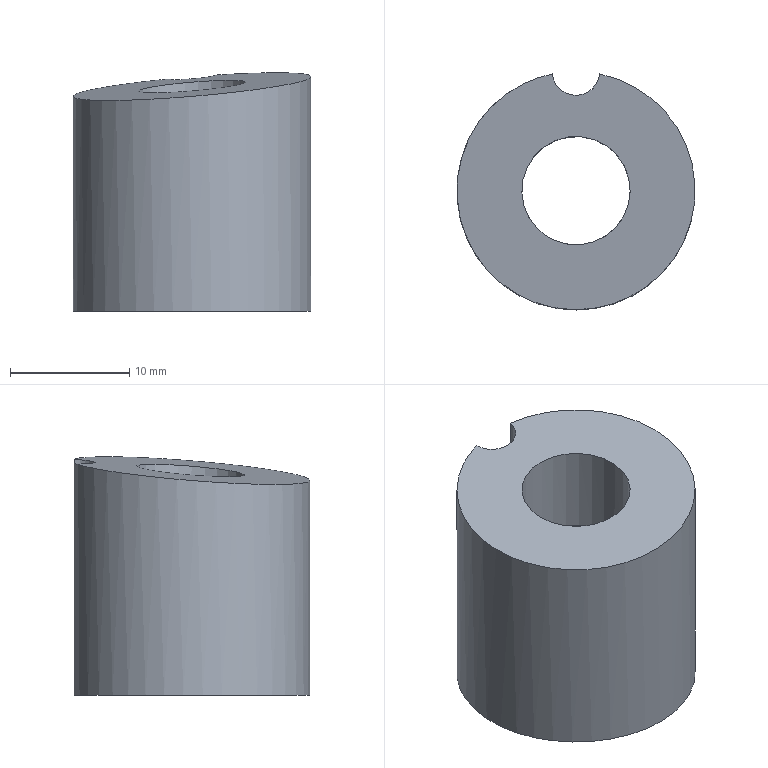Part | NX | features EKSD 20-20-10.10 2 | 1 solid | 7 faces | box 20 x 19.8 x 20.027 mm | volume 3866 mm3 | cylinder 4 | plane 3 | commonest cylinder face diameters 4 x1 9.1 x1 12.6 x1 20 x1
STEP:
#1=CARTESIAN_POINT('',(716.324,18.77,-15.));
#2=VERTEX_POINT('',#1);
#3=CARTESIAN_POINT('',(720.304,18.77,-15.));
#4=VERTEX_POINT('',#3);
#5=CARTESIAN_POINT('',(718.314,18.97,-15.));
#6=DIRECTION('',(0.,0.,1.));
#7=DIRECTION('',(1.,0.,0.));
#8=AXIS2_PLACEMENT_3D('',#5,#6,#7);
#9=CIRCLE('',#8,2.);
#10=EDGE_CURVE('',#2,#4,#9,.T.);
#11=ORIENTED_EDGE('',*,*,#10,.T.);
#12=CARTESIAN_POINT('',(718.314,8.97,-15.));
#13=DIRECTION('',(0.,0.,1.));
#14=DIRECTION('',(1.,0.,0.));
#15=AXIS2_PLACEMENT_3D('',#12,#13,#14);
#16=CIRCLE('',#15,10.);
#17=EDGE_CURVE('',#2,#4,#16,.T.);
#18=ORIENTED_EDGE('',*,*,#17,.F.);
#19=EDGE_LOOP('',(#11,#18));
#20=FACE_BOUND('',#19,.T.);
#21=CARTESIAN_POINT('',(712.014,8.97,-15.));
#22=VERTEX_POINT('',#21);
#23=CARTESIAN_POINT('',(718.314,8.97,-15.));
#24=DIRECTION('',(0.,0.,-1.));
#25=DIRECTION('',(-1.,0.,0.));
#26=AXIS2_PLACEMENT_3D('',#23,#24,#25);
#27=CIRCLE('',#26,6.3);
#28=EDGE_CURVE('',#22,#22,#27,.T.);
#29=ORIENTED_EDGE('',*,*,#28,.F.);
#30=EDGE_LOOP('',(#29));
#31=FACE_BOUND('',#30,.T.);
#32=CARTESIAN_POINT('',(718.314,8.97,-15.));
#33=DIRECTION('',(0.,0.,-1.));
#34=DIRECTION('',(-1.,0.,0.));
#35=AXIS2_PLACEMENT_3D('',#32,#33,#34);
#36=PLANE('',#35);
#37=ADVANCED_FACE('',(#20,#31),#36,.T.);
#38=CARTESIAN_POINT('',(720.304,18.77,4.83));
#39=VERTEX_POINT('',#38);
#40=CARTESIAN_POINT('',(716.324,18.77,4.501));
#41=VERTEX_POINT('',#40);
#42=CARTESIAN_POINT('',(718.314,18.97,4.682));
#43=DIRECTION('',(0.08207,0.08131,-0.9933));
#44=DIRECTION('',(-0.7057,-0.6991,-0.1155));
#45=AXIS2_PLACEMENT_3D('',#42,#43,#44);
#46=ELLIPSE('',#45,2.013,2.);
#47=EDGE_CURVE('',#39,#41,#46,.T.);
#48=ORIENTED_EDGE('',*,*,#47,.T.);
#49=CARTESIAN_POINT('',(718.314,8.97,3.864));
#50=DIRECTION('',(0.08207,0.08131,-0.9933));
#51=DIRECTION('',(-0.7057,-0.6991,-0.1155));
#52=AXIS2_PLACEMENT_3D('',#49,#50,#51);
#53=ELLIPSE('',#52,10.067,10.);
#54=EDGE_CURVE('',#39,#41,#53,.T.);
#55=ORIENTED_EDGE('',*,*,#54,.F.);
#56=EDGE_LOOP('',(#48,#55));
#57=FACE_BOUND('',#56,.T.);
#58=CARTESIAN_POINT('',(715.082,5.767,3.334));
#59=VERTEX_POINT('',#58);
#60=CARTESIAN_POINT('',(718.314,8.97,3.864));
#61=DIRECTION('',(0.08207,0.08131,-0.9933));
#62=DIRECTION('',(-0.7057,-0.6991,-0.1155));
#63=AXIS2_PLACEMENT_3D('',#60,#61,#62);
#64=ELLIPSE('',#63,4.581,4.55);
#65=EDGE_CURVE('',#59,#59,#64,.F.);
#66=ORIENTED_EDGE('',*,*,#65,.F.);
#67=EDGE_LOOP('',(#66));
#68=FACE_BOUND('',#67,.T.);
#69=CARTESIAN_POINT('',(769.706,-95.382,-0.4319));
#70=DIRECTION('',(0.08207,0.08131,-0.9933));
#71=DIRECTION('',(0.9966,-0.01117,0.08143));
#72=AXIS2_PLACEMENT_3D('',#69,#70,#71);
#73=PLANE('',#72);
#74=ADVANCED_FACE('',(#57,#68),#73,.F.);
#75=CARTESIAN_POINT('',(720.304,18.77,-5.));
#76=DIRECTION('',(0.,0.,-1.));
#77=VECTOR('',#76,1000.);
#78=LINE('',#75,#77);
#79=EDGE_CURVE('',#39,#4,#78,.T.);
#80=ORIENTED_EDGE('',*,*,#79,.F.);
#81=ORIENTED_EDGE('',*,*,#54,.T.);
#82=CARTESIAN_POINT('',(716.324,18.77,-5.));
#83=DIRECTION('',(0.,0.,-1.));
#84=VECTOR('',#83,1000.);
#85=LINE('',#82,#84);
#86=EDGE_CURVE('',#2,#41,#85,.F.);
#87=ORIENTED_EDGE('',*,*,#86,.F.);
#88=ORIENTED_EDGE('',*,*,#17,.T.);
#89=EDGE_LOOP('',(#80,#81,#87,#88));
#90=FACE_BOUND('',#89,.T.);
#91=CARTESIAN_POINT('',(718.314,8.97,5.));
#92=DIRECTION('',(0.,0.,-1.));
#93=DIRECTION('',(-1.,0.,0.));
#94=AXIS2_PLACEMENT_3D('',#91,#92,#93);
#95=CYLINDRICAL_SURFACE('',#94,10.);
#96=ADVANCED_FACE('',(#90),#95,.T.);
#97=CARTESIAN_POINT('',(722.864,8.97,-3.));
#98=VERTEX_POINT('',#97);
#99=CARTESIAN_POINT('',(718.314,8.97,-3.));
#100=DIRECTION('',(0.,0.,1.));
#101=DIRECTION('',(1.,0.,0.));
#102=AXIS2_PLACEMENT_3D('',#99,#100,#101);
#103=CIRCLE('',#102,4.55);
#104=EDGE_CURVE('',#98,#98,#103,.F.);
#105=ORIENTED_EDGE('',*,*,#104,.T.);
#106=EDGE_LOOP('',(#105));
#107=FACE_BOUND('',#106,.T.);
#108=ORIENTED_EDGE('',*,*,#65,.T.);
#109=EDGE_LOOP('',(#108));
#110=FACE_BOUND('',#109,.T.);
#111=CARTESIAN_POINT('',(718.314,8.97,6.));
#112=DIRECTION('',(0.,0.,-1.));
#113=DIRECTION('',(-1.,0.,0.));
#114=AXIS2_PLACEMENT_3D('',#111,#112,#113);
#115=CYLINDRICAL_SURFACE('',#114,4.55);
#116=ADVANCED_FACE('',(#107,#110),#115,.F.);
#117=CARTESIAN_POINT('',(712.014,8.97,-3.));
#118=VERTEX_POINT('',#117);
#119=CARTESIAN_POINT('',(718.314,8.97,-3.));
#120=DIRECTION('',(0.,0.,-1.));
#121=DIRECTION('',(-1.,0.,0.));
#122=AXIS2_PLACEMENT_3D('',#119,#120,#121);
#123=CIRCLE('',#122,6.3);
#124=EDGE_CURVE('',#118,#118,#123,.T.);
#125=ORIENTED_EDGE('',*,*,#124,.T.);
#126=EDGE_LOOP('',(#125));
#127=FACE_BOUND('',#126,.T.);
#128=ORIENTED_EDGE('',*,*,#104,.F.);
#129=EDGE_LOOP('',(#128));
#130=FACE_BOUND('',#129,.T.);
#131=CARTESIAN_POINT('',(718.314,8.97,-3.));
#132=DIRECTION('',(0.,0.,1.));
#133=DIRECTION('',(1.,0.,0.));
#134=AXIS2_PLACEMENT_3D('',#131,#132,#133);
#135=PLANE('',#134);
#136=ADVANCED_FACE('',(#127,#130),#135,.F.);
#137=ORIENTED_EDGE('',*,*,#28,.T.);
#138=EDGE_LOOP('',(#137));
#139=FACE_BOUND('',#138,.T.);
#140=ORIENTED_EDGE('',*,*,#124,.F.);
#141=EDGE_LOOP('',(#140));
#142=FACE_BOUND('',#141,.T.);
#143=CARTESIAN_POINT('',(718.314,8.97,-3.));
#144=DIRECTION('',(0.,0.,-1.));
#145=DIRECTION('',(-1.,0.,0.));
#146=AXIS2_PLACEMENT_3D('',#143,#144,#145);
#147=CYLINDRICAL_SURFACE('',#146,6.3);
#148=ADVANCED_FACE('',(#139,#142),#147,.F.);
#149=ORIENTED_EDGE('',*,*,#79,.T.);
#150=ORIENTED_EDGE('',*,*,#10,.F.);
#151=ORIENTED_EDGE('',*,*,#86,.T.);
#152=ORIENTED_EDGE('',*,*,#47,.F.);
#153=EDGE_LOOP('',(#149,#150,#151,#152));
#154=FACE_BOUND('',#153,.T.);
#155=CARTESIAN_POINT('',(718.314,18.97,5.));
#156=DIRECTION('',(0.,0.,-1.));
#157=DIRECTION('',(-1.,0.,0.));
#158=AXIS2_PLACEMENT_3D('',#155,#156,#157);
#159=CYLINDRICAL_SURFACE('',#158,2.);
#160=ADVANCED_FACE('',(#154),#159,.F.);
#161=CLOSED_SHELL('',(#37,#74,#96,#116,#136,#148,#160));
#162=MANIFOLD_SOLID_BREP('',#161);
#163=(LENGTH_UNIT()NAMED_UNIT(*)SI_UNIT(.MILLI.,.METRE.));
#164=UNCERTAINTY_MEASURE_WITH_UNIT(LENGTH_MEASURE(0.00001),#163,'','');
#165=(NAMED_UNIT(*)PLANE_ANGLE_UNIT()SI_UNIT($,.RADIAN.));
#166=(NAMED_UNIT(*)SI_UNIT($,.STERADIAN.)SOLID_ANGLE_UNIT());
#167=(GEOMETRIC_REPRESENTATION_CONTEXT(3)GLOBAL_UNCERTAINTY_ASSIGNED_CONTEXT((#164))GLOBAL_UNIT_ASSIGNED_CONTEXT((#163,#165,#166))REPRESENTATION_CONTEXT('',''));
#168=ADVANCED_BREP_SHAPE_REPRESENTATION('',(#162),#167);